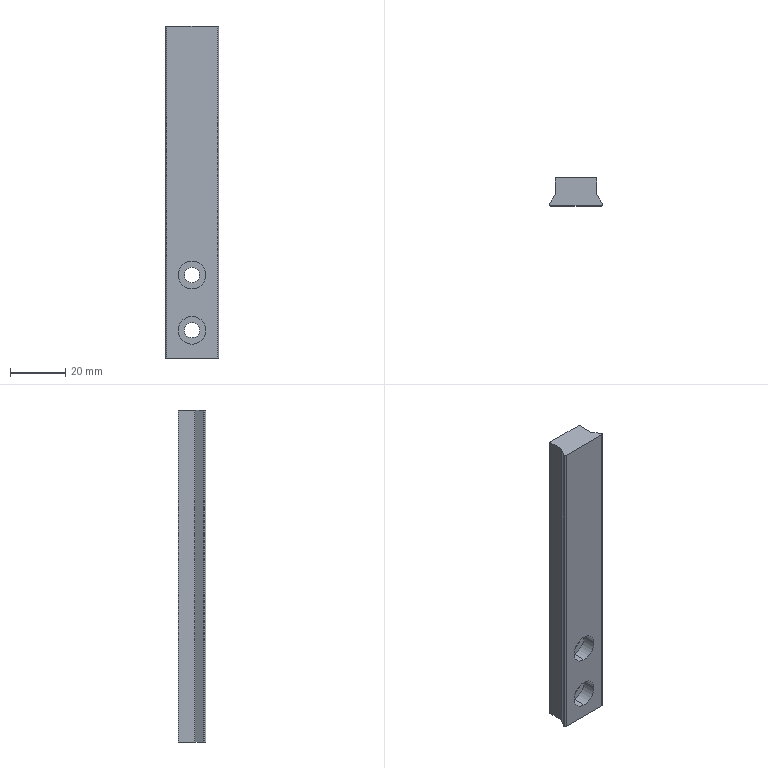Part | STEP file | slider 2 | 1 solid | 21 faces | box 19.196 x 10 x 120 mm | volume 18133 mm3 | cylinder 11 | plane 10 | commonest cylinder face diameters 5.5 x4 10 x4 1 x3